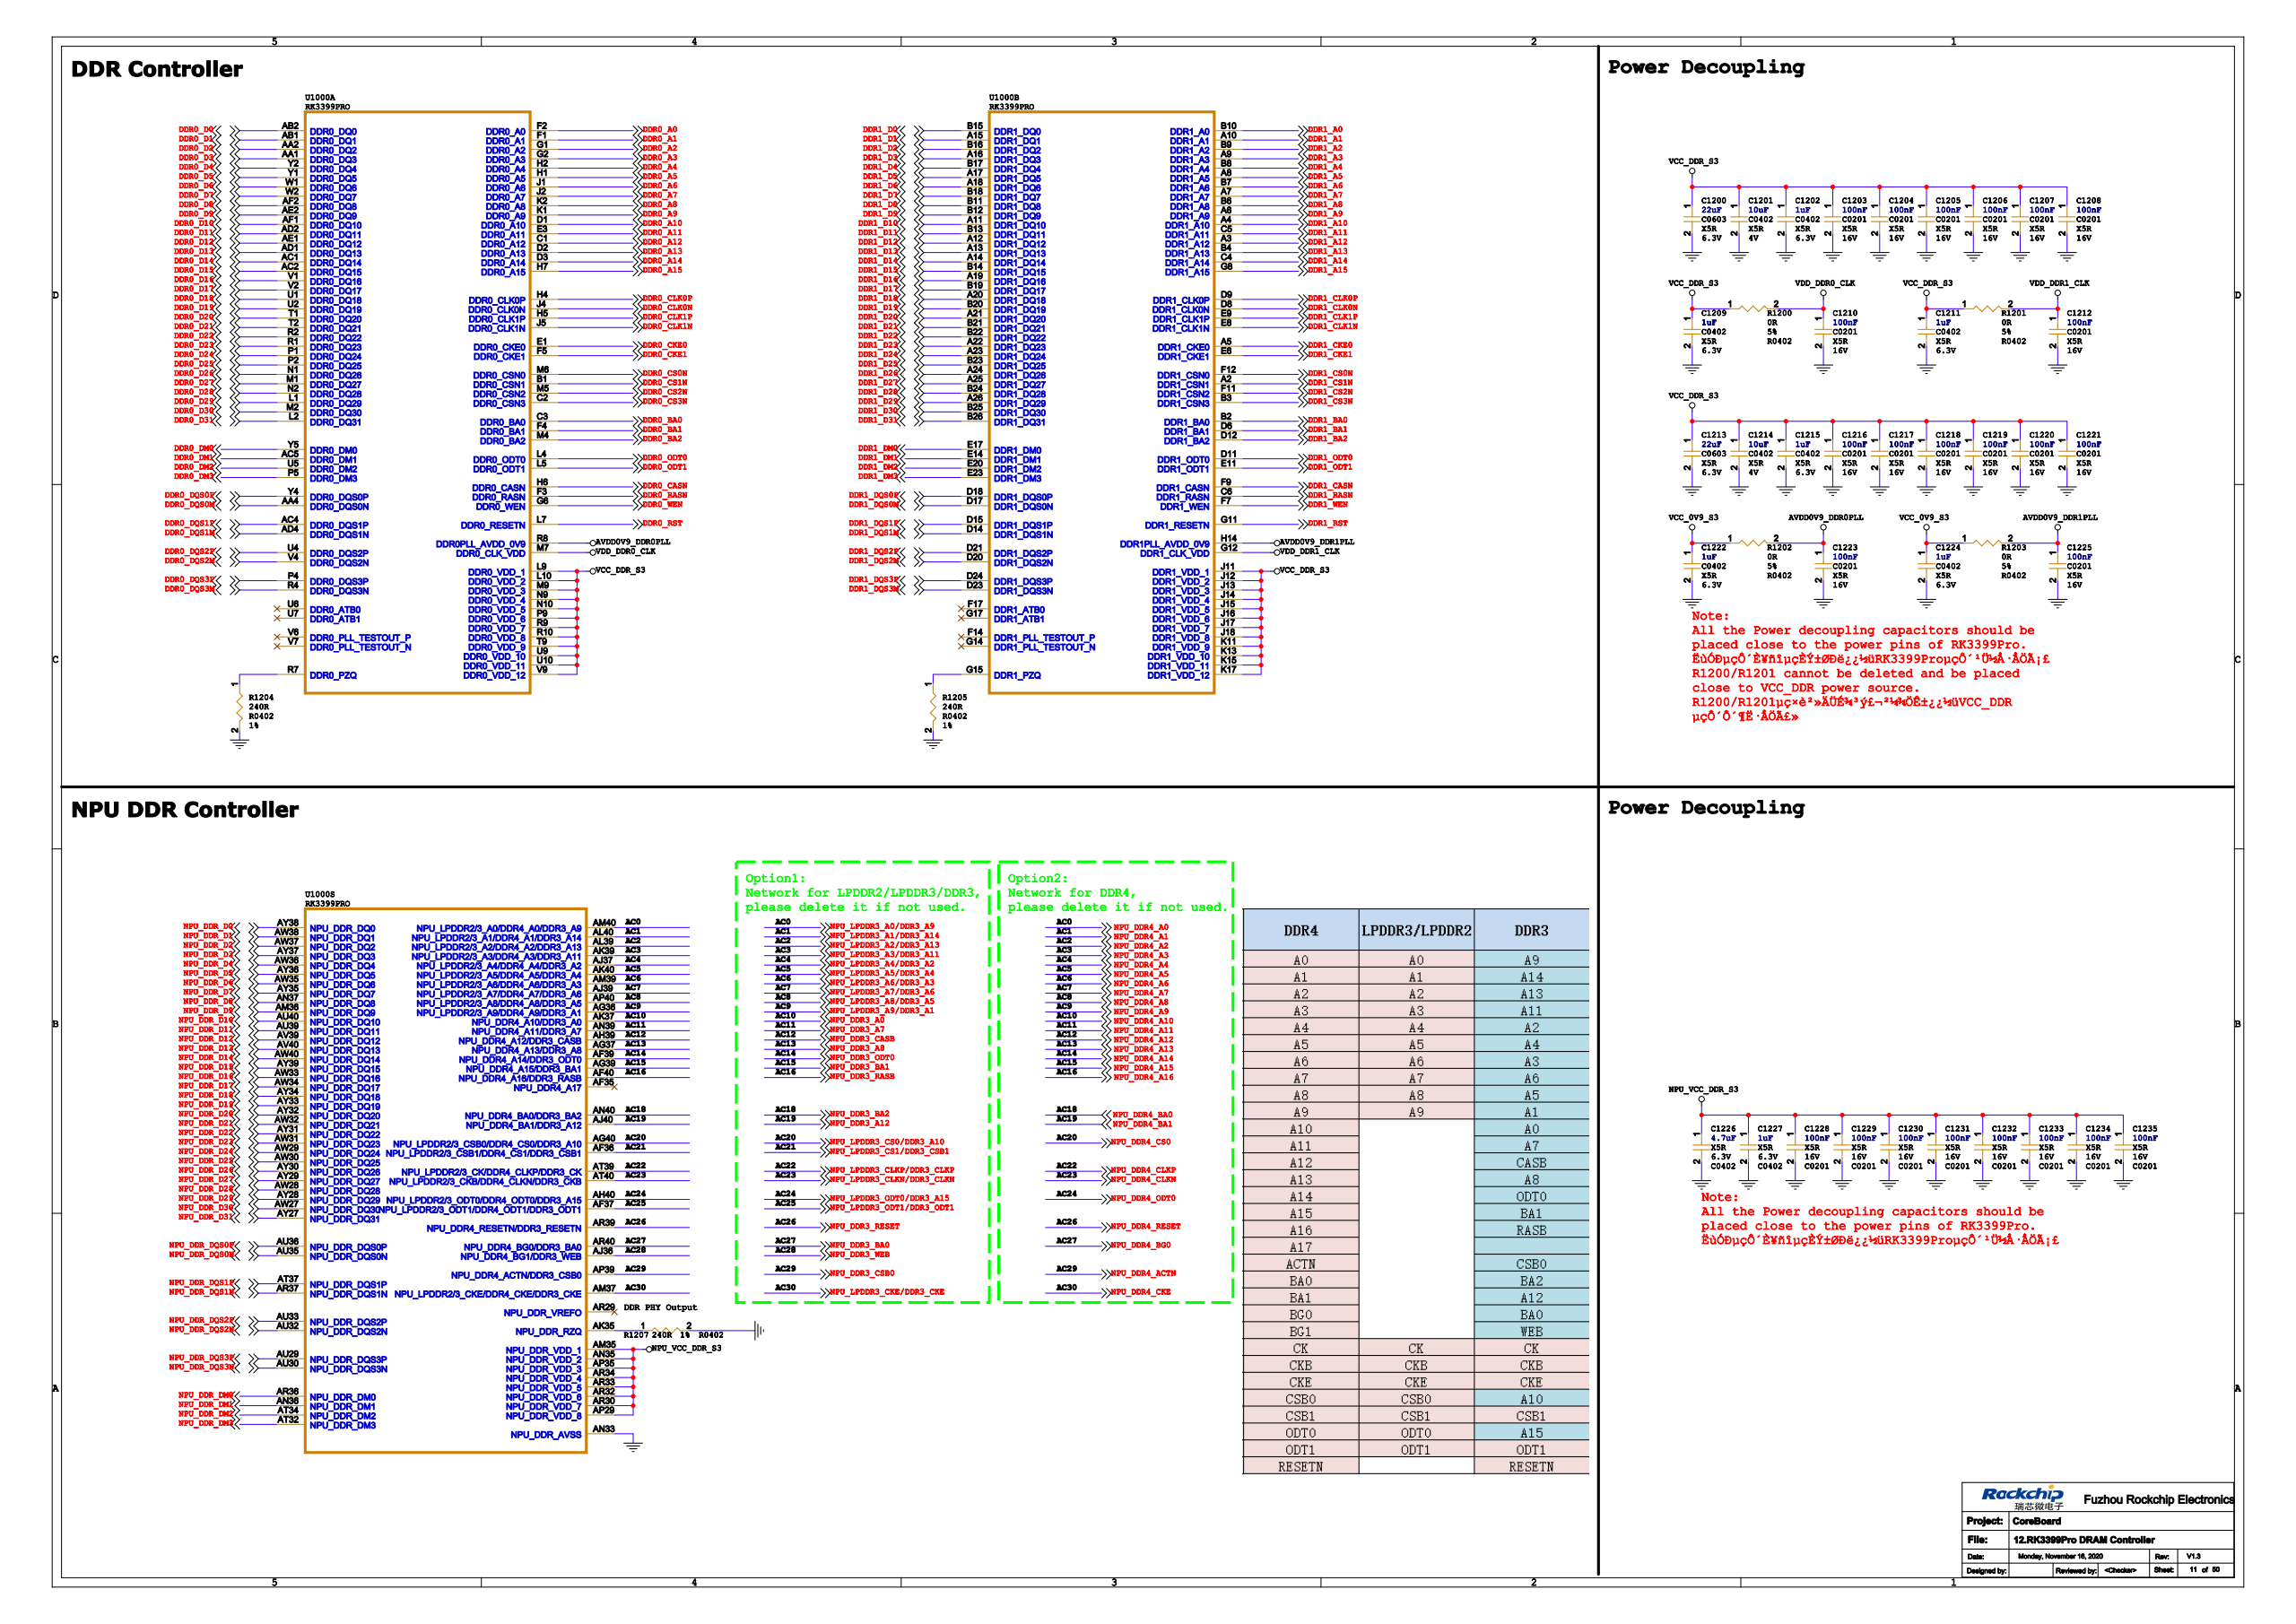Circuit board | Cadence Allegro | 749 parts | 717 nets | one sheet of the schematic
Parts on this sheet (reference | value | footprint):
C1200 | 22uF | C0603
C1201 | 10uF | C0402
C1202 | 1uF | C0402
C1203 | 100nF | C0201
C1204 | 100nF | C0201
C1205 | 100nF | C0201
C1206 | 100nF | C0201
C1207 | 100nF | C0201
C1208 | 100nF | C0201
C1209 | 1uF | C0402
C1210 | 100nF | C0201
C1211 | 1uF | C0402
C1212 | 100nF | C0201
C1213 | 22uF | C0603
C1214 | 10uF | C0402
C1215 | 1uF | C0402
C1216 | 100nF | C0201
C1217 | 100nF | C0201
C1218 | 100nF | C0201
C1219 | 100nF | C0201
C1220 | 100nF | C0201
C1221 | 100nF | C0201
C1222 | 1uF | C0402
C1223 | 100nF | C0201
C1224 | 1uF | C0402
C1225 | 100nF | C0201
C1226 | 4.7uF | C0402
C1227 | 1uF | C0402
C1228 | 100nF | C0201
C1229 | 100nF | C0201
C1230 | 100nF | C0201
C1231 | 100nF | C0201
C1232 | 100nF | C0201
C1233 | 100nF | C0201
C1234 | 100nF | C0201
C1235 | 100nF | C0201
R1200 | 0R | R0402
R1201 | 0R | R0402
R1202 | 0R | R0402
R1203 | 0R | R0402
R1204 | 240R | R0402
R1205 | 240R | R0402
R1207 | 240R | R0402
U1000 | RK3399PRO | BGA1372_27R00X27R00X2R19
Nets of these parts (net: part-pin ...):
GND: C1200-2 C1201-2 C1202-2 C1203-2 C1204-2 C1205-2 C1206-2 C1207-2 C1208-2 C1209-2 C1210-2 C1211-2 C1212-2 C1213-2 C1214-2 C1215-2 C1216-2 C1217-2 C1218-2 C1219-2 C1220-2 C1221-2 C1222-2 C1223-2 C1224-2 C1225-2 C1226-2 C1227-2 C1228-2 C1229-2 C1230-2 C1231-2 C1232-2 C1233-2 C1234-2 C1235-2 R1204-2 R1205-2 R1207-2 U1000-AC3 U1000-AC11 U1000-AC13 U1000-AC15 U1000-AC16 U1000-AC18 U1000-AC19 U1000-AC20 U1000-AC21 U1000-AC22 U1000-AC23 U1000-AC25 U1000-AC26 U1000-AN33
VCC_DDR_S3: C1200-1 C1201-1 C1202-1 C1203-1 C1204-1 C1205-1 C1206-1 C1207-1 C1208-1 C1209-1 C1211-1 C1213-1 C1214-1 C1215-1 C1216-1 C1217-1 C1218-1 C1219-1 C1220-1 C1221-1 R1200-1 R1201-1 U1000-J11 U1000-J12 U1000-J13 U1000-J14 U1000-J15 U1000-J16 U1000-J17 U1000-J18 U1000-K11 U1000-K13 U1000-K15 U1000-K17 U1000-L9 U1000-L10 U1000-M9 U1000-N9 U1000-N10 U1000-P9 U1000-R9 U1000-R10 U1000-T9 U1000-U9 U1000-U10 U1000-V9
NPU_VCC_DDR_S3: C1226-1 C1227-1 C1228-1 C1229-1 C1230-1 C1231-1 C1232-1 C1233-1 C1234-1 C1235-1 U1000-AM35 U1000-AN35 U1000-AP29 U1000-AP35 U1000-AR30 U1000-AR32 U1000-AR33 U1000-AR34
AVDD0V9_DDR0PLL: C1223-1 R1202-2 U1000-R8
DDR0_A0: U1000-F2
DDR0_A1: U1000-F1
DDR0_A10: U1000-D1
DDR0_A11: U1000-E3
DDR0_A12: U1000-C1
DDR0_A13: U1000-D2
DDR0_A14: U1000-D3
DDR0_A15: U1000-H7
DDR0_A2: U1000-G1
DDR0_A3: U1000-G2
DDR0_A4: U1000-H2
DDR0_A5: U1000-H1
DDR0_A6: U1000-J1
DDR0_A7: U1000-J2
DDR0_A8: U1000-K2
DDR0_A9: U1000-K1
DDR0_BA0: U1000-C3
DDR0_BA1: U1000-F4
DDR0_BA2: U1000-M4
DDR0_CASN: U1000-H6
DDR0_CKE0: U1000-E1
DDR0_CKE1: U1000-F5
DDR0_CLK0N: U1000-J4
DDR0_CLK0P: U1000-H4
DDR0_CLK1N: U1000-J5
DDR0_CLK1P: U1000-H5
VDD_DDR0_CLK: C1210-1 R1200-2 U1000-M7
DDR0_CS0N: U1000-M6
DDR0_CS1N: U1000-B1
DDR0_CS2N: U1000-M5
DDR0_CS3N: U1000-C2
DDR0_DM0: U1000-Y5
DDR0_DM1: U1000-AC5
DDR0_DM2: U1000-U5
DDR0_DM3: U1000-P5
DDR0_D0: U1000-AB2
DDR0_D1: U1000-AB1
DDR0_D10: U1000-AF1
DDR0_D11: U1000-AD2
DDR0_D12: U1000-AE1
DDR0_D13: U1000-AD1
DDR0_D14: U1000-AC1
DDR0_D15: U1000-AC2
DDR0_D16: U1000-V1
DDR0_D17: U1000-V2
DDR0_D18: U1000-U1
DDR0_D19: U1000-U2
DDR0_D2: U1000-AA2
DDR0_D20: U1000-T1
DDR0_D21: U1000-T2
DDR0_D22: U1000-R2
DDR0_D23: U1000-R1
DDR0_D24: U1000-P1
DDR0_D25: U1000-P2
DDR0_D26: U1000-N1
DDR0_D27: U1000-M1
DDR0_D28: U1000-N2
DDR0_D29: U1000-L1
DDR0_D3: U1000-AA1
DDR0_D30: U1000-M2
DDR0_D31: U1000-L2
DDR0_D4: U1000-Y2
DDR0_D5: U1000-Y1
DDR0_D6: U1000-W1
DDR0_D7: U1000-W2
DDR0_D8: U1000-AF2
DDR0_D9: U1000-AE2
DDR0_DQS0M: U1000-AA4
DDR0_DQS0P: U1000-Y4
DDR0_DQS1M: U1000-AD4
DDR0_DQS1P: U1000-AC4
DDR0_DQS2M: U1000-V4
DDR0_DQS2P: U1000-U4
DDR0_DQS3M: U1000-R4
DDR0_DQS3P: U1000-P4
DDR0_ODT0: U1000-L4
DDR0_ODT1: U1000-L5
N78239852: R1204-1 U1000-R7
DDR0_RASN: U1000-F3
DDR0_RST: U1000-L7
DDR0_WEN: U1000-G6
AVDD0V9_DDR1PLL: C1225-1 R1203-2 U1000-H14
DDR1_A0: U1000-B10
DDR1_A1: U1000-A10
DDR1_A10: U1000-A4
DDR1_A11: U1000-C5
DDR1_A12: U1000-A3
DDR1_A13: U1000-B4
DDR1_A14: U1000-C4
DDR1_A15: U1000-G8
DDR1_A2: U1000-B9
DDR1_A3: U1000-A9
DDR1_A4: U1000-B8
DDR1_A5: U1000-A8
DDR1_A6: U1000-B7
DDR1_A7: U1000-A7
DDR1_A8: U1000-B6
DDR1_A9: U1000-A6
DDR1_BA0: U1000-B2
DDR1_BA1: U1000-D6
DDR1_BA2: U1000-D12
DDR1_CASN: U1000-F9
DDR1_CKE0: U1000-A5
DDR1_CKE1: U1000-E6
DDR1_CLK0N: U1000-D8
DDR1_CLK0P: U1000-D9
DDR1_CLK1N: U1000-E8
DDR1_CLK1P: U1000-E9
VDD_DDR1_CLK: C1212-1 R1201-2 U1000-G12
DDR1_CS0N: U1000-F12
DDR1_CS1N: U1000-A2
DDR1_CS2N: U1000-F11
DDR1_CS3N: U1000-B3
DDR1_DM0: U1000-E17
DDR1_DM1: U1000-E14
DDR1_DM2: U1000-E20
DDR1_DM3: U1000-E23
DDR1_D0: U1000-B15
DDR1_D1: U1000-A15
DDR1_D10: U1000-A11
DDR1_D11: U1000-B13
DDR1_D12: U1000-A12
DDR1_D13: U1000-A13
DDR1_D14: U1000-A14
DDR1_D15: U1000-B14
DDR1_D16: U1000-A19
DDR1_D17: U1000-B19
DDR1_D18: U1000-A20
DDR1_D19: U1000-B20
DDR1_D2: U1000-B16
DDR1_D20: U1000-A21
DDR1_D21: U1000-B21
DDR1_D22: U1000-B22
DDR1_D23: U1000-A22
DDR1_D24: U1000-A23
DDR1_D25: U1000-B23
DDR1_D26: U1000-A24
DDR1_D27: U1000-A25
DDR1_D28: U1000-B24
DDR1_D29: U1000-A26
DDR1_D3: U1000-A16
DDR1_D30: U1000-B25
DDR1_D31: U1000-B26
DDR1_D4: U1000-B17
DDR1_D5: U1000-A17
DDR1_D6: U1000-A18
DDR1_D7: U1000-B18
DDR1_D8: U1000-B11
DDR1_D9: U1000-B12
DDR1_DQS0M: U1000-D17
DDR1_DQS0P: U1000-D18
DDR1_DQS1M: U1000-D14
DDR1_DQS1P: U1000-D15
DDR1_DQS2M: U1000-D20
DDR1_DQS2P: U1000-D21
DDR1_DQS3M: U1000-D23
DDR1_DQS3P: U1000-D24
DDR1_ODT0: U1000-D11
DDR1_ODT1: U1000-E11
N78245073: R1205-1 U1000-G15
DDR1_RASN: U1000-C6
DDR1_RST: U1000-G11
DDR1_WEN: U1000-F7
VCC_0V9_S3: C1222-1 C1224-1 R1202-1 R1203-1
NPU_DDR3_A0: U1000-AK37
NPU_DDR3_A12: U1000-AJ40
NPU_DDR3_A7: U1000-AN39
NPU_DDR3_A8: U1000-AG37
NPU_DDR3_BA0: U1000-AR40
NPU_DDR3_BA1: U1000-AG39
NPU_DDR3_BA2: U1000-AN40
NPU_DDR3_CASB: U1000-AH39
NPU_DDR3_CSB0: U1000-AP39
NPU_DDR3_ODT0: U1000-AF39
NPU_DDR3_RASB: U1000-AF40
NPU_DDR3_RESET: U1000-AR39
NPU_DDR3_WEB: U1000-AJ36
NPU_DDR_DM0: U1000-AR36
NPU_DDR_DM1: U1000-AN36
NPU_DDR_DM2: U1000-AT34
NPU_DDR_DM3: U1000-AT32
NPU_DDR_D0: U1000-AY38
NPU_DDR_D1: U1000-AW38
NPU_DDR_D10: U1000-AU40
NPU_DDR_D11: U1000-AU39
NPU_DDR_D12: U1000-AV39
NPU_DDR_D13: U1000-AV40
NPU_DDR_D14: U1000-AW40
NPU_DDR_D15: U1000-AY39
NPU_DDR_D16: U1000-AW33
NPU_DDR_D17: U1000-AW34
NPU_DDR_D18: U1000-AY34
NPU_DDR_D19: U1000-AY33
NPU_DDR_D2: U1000-AW37
NPU_DDR_D20: U1000-AY32
NPU_DDR_D21: U1000-AW32
NPU_DDR_D22: U1000-AY31
NPU_DDR_D23: U1000-AW31
NPU_DDR_D24: U1000-AW29
NPU_DDR_D25: U1000-AW30
NPU_DDR_D26: U1000-AY30
NPU_DDR_D27: U1000-AY29
NPU_DDR_D28: U1000-AW28
NPU_DDR_D29: U1000-AY28
NPU_DDR_D3: U1000-AY37
NPU_DDR_D30: U1000-AW27
NPU_DDR_D31: U1000-AY27
NPU_DDR_D4: U1000-AW36
NPU_DDR_D5: U1000-AY36
NPU_DDR_D6: U1000-AW35
NPU_DDR_D7: U1000-AY35
NPU_DDR_D8: U1000-AN37
NPU_DDR_D9: U1000-AM36
NPU_DDR_DQS0N: U1000-AU35
NPU_DDR_DQS0P: U1000-AU36
NPU_DDR_DQS1N: U1000-AR37
NPU_DDR_DQS1P: U1000-AT37
NPU_DDR_DQS2N: U1000-AU32
NPU_DDR_DQS2P: U1000-AU33
NPU_DDR_DQS3N: U1000-AU30
NPU_DDR_DQS3P: U1000-AU29
N78331808: R1207-1 U1000-AK35
NPU_DDR4_A0: U1000-AM40
NPU_DDR4_A1: U1000-AL40
NPU_DDR4_A2: U1000-AL39
NPU_DDR4_A3: U1000-AK39
NPU_DDR4_A4: U1000-AJ37
NPU_DDR4_A5: U1000-AK40
NPU_DDR4_A6: U1000-AM39
NPU_DDR4_A7: U1000-AJ39
NPU_DDR4_A8: U1000-AP40
NPU_DDR4_A9: U1000-AG36
NPU_DDR4_CKE: U1000-AM37
NPU_DDR4_CLKP: U1000-AT39
NPU_DDR4_CLKN: U1000-AT40
NPU_DDR4_CS0: U1000-AG40
NPU_LPDDR3_CS1/DDR3_CSB1: U1000-AF36
NPU_DDR4_ODT0: U1000-AH40
NPU_LPDDR3_ODT1/DDR3_ODT1: U1000-AF37